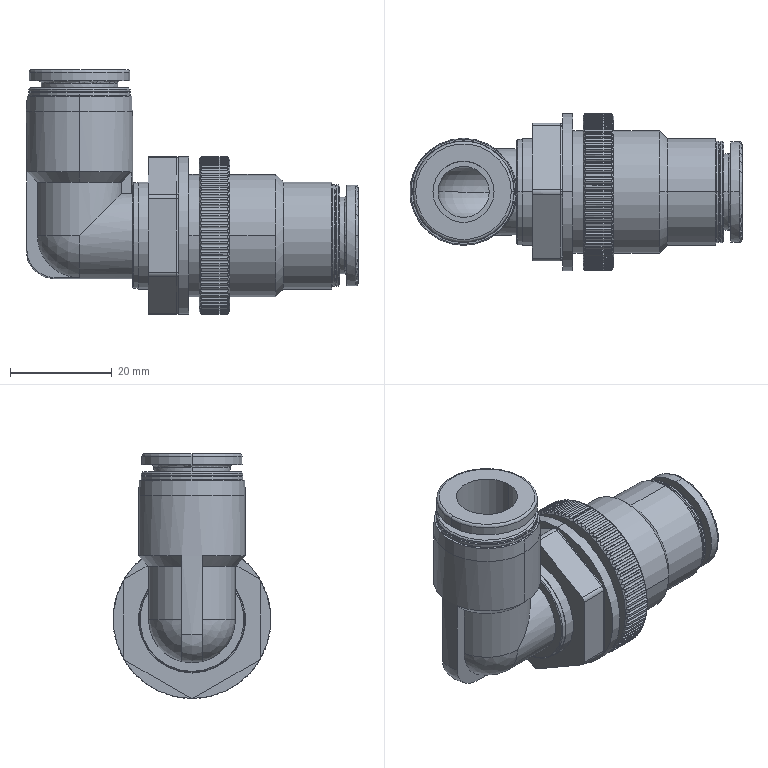Part | SolidWorks | features BaseBody 1 | 1 solid | 349 faces | box 65.2 x 31 x 48.1 mm | volume 24848 mm3 | cylinder 272 | cone 29 | plane 27 | torus 18 | sphere 2 | spline 1 | commonest cylinder face diameters 0.659 x131 31 x90 20 x8 2 x7 1 x6 21 x6